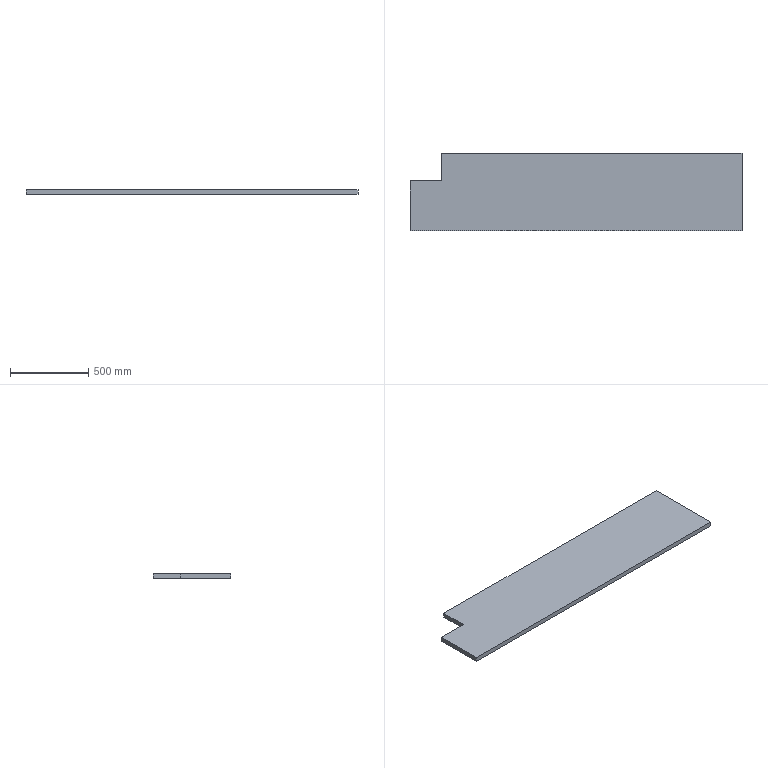Part | SolidWorks | features 3DProfileFeature 1, Extrusion 1, HoleWzd 1 | 1 solid | 24 faces | box 2118 x 492 x 30 mm | volume 30183108 mm3 | cylinder 8 | cone 8 | plane 8 | commonest cylinder face diameters 14 x8
STEP:
#1=CARTESIAN_POINT('',(918.,447.,8.));
#2=VERTEX_POINT('',#1);
#3=CARTESIAN_POINT('',(918.,447.,22.));
#4=VERTEX_POINT('',#3);
#5=CARTESIAN_POINT('',(918.,447.,15.));
#6=DIRECTION('',(0.,1.,0.));
#7=DIRECTION('',(0.,0.,1.));
#8=AXIS2_PLACEMENT_3D('',#5,#6,#7);
#9=CIRCLE('',#8,7.);
#10=EDGE_CURVE('',#2,#4,#9,.T.);
#11=ORIENTED_EDGE('',*,*,#10,.F.);
#12=CARTESIAN_POINT('',(918.,492.,8.));
#13=VERTEX_POINT('',#12);
#14=CARTESIAN_POINT('',(918.,492.,8.));
#15=DIRECTION('',(0.,1.,0.));
#16=VECTOR('',#15,1000.);
#17=LINE('',#14,#16);
#18=EDGE_CURVE('',#2,#13,#17,.T.);
#19=ORIENTED_EDGE('',*,*,#18,.T.);
#20=CARTESIAN_POINT('',(918.,492.,22.));
#21=VERTEX_POINT('',#20);
#22=CARTESIAN_POINT('',(918.,492.,15.));
#23=DIRECTION('',(0.,1.,0.));
#24=DIRECTION('',(0.,0.,1.));
#25=AXIS2_PLACEMENT_3D('',#22,#23,#24);
#26=CIRCLE('',#25,7.);
#27=EDGE_CURVE('',#13,#21,#26,.T.);
#28=ORIENTED_EDGE('',*,*,#27,.T.);
#29=CARTESIAN_POINT('',(918.,492.,22.));
#30=DIRECTION('',(0.,1.,0.));
#31=VECTOR('',#30,1000.);
#32=LINE('',#29,#31);
#33=EDGE_CURVE('',#4,#21,#32,.T.);
#34=ORIENTED_EDGE('',*,*,#33,.F.);
#35=EDGE_LOOP('',(#11,#19,#28,#34));
#36=FACE_OUTER_BOUND('',#35,.T.);
#37=CARTESIAN_POINT('',(918.,492.,15.));
#38=DIRECTION('',(0.,1.,0.));
#39=DIRECTION('',(0.,0.,1.));
#40=AXIS2_PLACEMENT_3D('',#37,#38,#39);
#41=CYLINDRICAL_SURFACE('',#40,7.);
#42=ADVANCED_FACE('',(#36),#41,.F.);
#43=CARTESIAN_POINT('',(918.,442.794,15.));
#44=VERTEX_POINT('',#43);
#45=CARTESIAN_POINT('',(918.,447.,22.));
#46=DIRECTION('',(0.,0.515,0.8572));
#47=VECTOR('',#46,1000.);
#48=LINE('',#45,#47);
#49=EDGE_CURVE('',#44,#4,#48,.T.);
#50=ORIENTED_EDGE('',*,*,#49,.F.);
#51=CARTESIAN_POINT('',(918.,447.,8.));
#52=DIRECTION('',(0.,0.515,-0.8572));
#53=VECTOR('',#52,1000.);
#54=LINE('',#51,#53);
#55=EDGE_CURVE('',#44,#2,#54,.T.);
#56=ORIENTED_EDGE('',*,*,#55,.T.);
#57=ORIENTED_EDGE('',*,*,#10,.T.);
#58=EDGE_LOOP('',(#50,#56,#57));
#59=FACE_OUTER_BOUND('',#58,.T.);
#60=CARTESIAN_POINT('',(918.,447.,15.));
#61=DIRECTION('',(0.,1.,0.));
#62=DIRECTION('',(0.,0.,1.));
#63=AXIS2_PLACEMENT_3D('',#60,#61,#62);
#64=CONICAL_SURFACE('',#63,7.,1.03);
#65=ADVANCED_FACE('',(#59),#64,.F.);
#66=CARTESIAN_POINT('',(1018.,447.,8.));
#67=VERTEX_POINT('',#66);
#68=CARTESIAN_POINT('',(1018.,447.,22.));
#69=VERTEX_POINT('',#68);
#70=CARTESIAN_POINT('',(1018.,447.,15.));
#71=DIRECTION('',(0.,1.,0.));
#72=DIRECTION('',(0.,0.,1.));
#73=AXIS2_PLACEMENT_3D('',#70,#71,#72);
#74=CIRCLE('',#73,7.);
#75=EDGE_CURVE('',#67,#69,#74,.T.);
#76=ORIENTED_EDGE('',*,*,#75,.F.);
#77=CARTESIAN_POINT('',(1018.,492.,8.));
#78=VERTEX_POINT('',#77);
#79=CARTESIAN_POINT('',(1018.,492.,8.));
#80=DIRECTION('',(0.,1.,0.));
#81=VECTOR('',#80,1000.);
#82=LINE('',#79,#81);
#83=EDGE_CURVE('',#67,#78,#82,.T.);
#84=ORIENTED_EDGE('',*,*,#83,.T.);
#85=CARTESIAN_POINT('',(1018.,492.,22.));
#86=VERTEX_POINT('',#85);
#87=CARTESIAN_POINT('',(1018.,492.,15.));
#88=DIRECTION('',(0.,1.,0.));
#89=DIRECTION('',(0.,0.,1.));
#90=AXIS2_PLACEMENT_3D('',#87,#88,#89);
#91=CIRCLE('',#90,7.);
#92=EDGE_CURVE('',#78,#86,#91,.T.);
#93=ORIENTED_EDGE('',*,*,#92,.T.);
#94=CARTESIAN_POINT('',(1018.,492.,22.));
#95=DIRECTION('',(0.,1.,0.));
#96=VECTOR('',#95,1000.);
#97=LINE('',#94,#96);
#98=EDGE_CURVE('',#69,#86,#97,.T.);
#99=ORIENTED_EDGE('',*,*,#98,.F.);
#100=EDGE_LOOP('',(#76,#84,#93,#99));
#101=FACE_OUTER_BOUND('',#100,.T.);
#102=CARTESIAN_POINT('',(1018.,492.,15.));
#103=DIRECTION('',(0.,1.,0.));
#104=DIRECTION('',(0.,0.,1.));
#105=AXIS2_PLACEMENT_3D('',#102,#103,#104);
#106=CYLINDRICAL_SURFACE('',#105,7.);
#107=ADVANCED_FACE('',(#101),#106,.F.);
#108=CARTESIAN_POINT('',(1018.,442.794,15.));
#109=VERTEX_POINT('',#108);
#110=CARTESIAN_POINT('',(1018.,447.,22.));
#111=DIRECTION('',(0.,0.515,0.8572));
#112=VECTOR('',#111,1000.);
#113=LINE('',#110,#112);
#114=EDGE_CURVE('',#109,#69,#113,.T.);
#115=ORIENTED_EDGE('',*,*,#114,.F.);
#116=CARTESIAN_POINT('',(1018.,447.,8.));
#117=DIRECTION('',(0.,0.515,-0.8572));
#118=VECTOR('',#117,1000.);
#119=LINE('',#116,#118);
#120=EDGE_CURVE('',#109,#67,#119,.T.);
#121=ORIENTED_EDGE('',*,*,#120,.T.);
#122=ORIENTED_EDGE('',*,*,#75,.T.);
#123=EDGE_LOOP('',(#115,#121,#122));
#124=FACE_OUTER_BOUND('',#123,.T.);
#125=CARTESIAN_POINT('',(1018.,447.,15.));
#126=DIRECTION('',(0.,1.,0.));
#127=DIRECTION('',(0.,0.,1.));
#128=AXIS2_PLACEMENT_3D('',#125,#126,#127);
#129=CONICAL_SURFACE('',#128,7.,1.03);
#130=ADVANCED_FACE('',(#124),#129,.F.);
#131=CARTESIAN_POINT('',(2068.,447.,8.));
#132=VERTEX_POINT('',#131);
#133=CARTESIAN_POINT('',(2068.,447.,22.));
#134=VERTEX_POINT('',#133);
#135=CARTESIAN_POINT('',(2068.,447.,15.));
#136=DIRECTION('',(0.,1.,0.));
#137=DIRECTION('',(0.,0.,1.));
#138=AXIS2_PLACEMENT_3D('',#135,#136,#137);
#139=CIRCLE('',#138,7.);
#140=EDGE_CURVE('',#132,#134,#139,.T.);
#141=ORIENTED_EDGE('',*,*,#140,.F.);
#142=CARTESIAN_POINT('',(2068.,492.,8.));
#143=VERTEX_POINT('',#142);
#144=CARTESIAN_POINT('',(2068.,492.,8.));
#145=DIRECTION('',(0.,1.,0.));
#146=VECTOR('',#145,1000.);
#147=LINE('',#144,#146);
#148=EDGE_CURVE('',#132,#143,#147,.T.);
#149=ORIENTED_EDGE('',*,*,#148,.T.);
#150=CARTESIAN_POINT('',(2068.,492.,22.));
#151=VERTEX_POINT('',#150);
#152=CARTESIAN_POINT('',(2068.,492.,15.));
#153=DIRECTION('',(0.,1.,0.));
#154=DIRECTION('',(0.,0.,1.));
#155=AXIS2_PLACEMENT_3D('',#152,#153,#154);
#156=CIRCLE('',#155,7.);
#157=EDGE_CURVE('',#143,#151,#156,.T.);
#158=ORIENTED_EDGE('',*,*,#157,.T.);
#159=CARTESIAN_POINT('',(2068.,492.,22.));
#160=DIRECTION('',(0.,1.,0.));
#161=VECTOR('',#160,1000.);
#162=LINE('',#159,#161);
#163=EDGE_CURVE('',#134,#151,#162,.T.);
#164=ORIENTED_EDGE('',*,*,#163,.F.);
#165=EDGE_LOOP('',(#141,#149,#158,#164));
#166=FACE_OUTER_BOUND('',#165,.T.);
#167=CARTESIAN_POINT('',(2068.,492.,15.));
#168=DIRECTION('',(0.,1.,0.));
#169=DIRECTION('',(0.,0.,1.));
#170=AXIS2_PLACEMENT_3D('',#167,#168,#169);
#171=CYLINDRICAL_SURFACE('',#170,7.);
#172=ADVANCED_FACE('',(#166),#171,.F.);
#173=CARTESIAN_POINT('',(2068.,442.794,15.));
#174=VERTEX_POINT('',#173);
#175=CARTESIAN_POINT('',(2068.,447.,22.));
#176=DIRECTION('',(0.,0.515,0.8572));
#177=VECTOR('',#176,1000.);
#178=LINE('',#175,#177);
#179=EDGE_CURVE('',#174,#134,#178,.T.);
#180=ORIENTED_EDGE('',*,*,#179,.F.);
#181=CARTESIAN_POINT('',(2068.,447.,8.));
#182=DIRECTION('',(0.,0.515,-0.8572));
#183=VECTOR('',#182,1000.);
#184=LINE('',#181,#183);
#185=EDGE_CURVE('',#174,#132,#184,.T.);
#186=ORIENTED_EDGE('',*,*,#185,.T.);
#187=ORIENTED_EDGE('',*,*,#140,.T.);
#188=EDGE_LOOP('',(#180,#186,#187));
#189=FACE_OUTER_BOUND('',#188,.T.);
#190=CARTESIAN_POINT('',(2068.,447.,15.));
#191=DIRECTION('',(0.,1.,0.));
#192=DIRECTION('',(0.,0.,1.));
#193=AXIS2_PLACEMENT_3D('',#190,#191,#192);
#194=CONICAL_SURFACE('',#193,7.,1.03);
#195=ADVANCED_FACE('',(#189),#194,.F.);
#196=CARTESIAN_POINT('',(1968.,447.,8.));
#197=VERTEX_POINT('',#196);
#198=CARTESIAN_POINT('',(1968.,447.,22.));
#199=VERTEX_POINT('',#198);
#200=CARTESIAN_POINT('',(1968.,447.,15.));
#201=DIRECTION('',(0.,1.,0.));
#202=DIRECTION('',(0.,0.,1.));
#203=AXIS2_PLACEMENT_3D('',#200,#201,#202);
#204=CIRCLE('',#203,7.);
#205=EDGE_CURVE('',#197,#199,#204,.T.);
#206=ORIENTED_EDGE('',*,*,#205,.F.);
#207=CARTESIAN_POINT('',(1968.,492.,8.));
#208=VERTEX_POINT('',#207);
#209=CARTESIAN_POINT('',(1968.,492.,8.));
#210=DIRECTION('',(0.,1.,0.));
#211=VECTOR('',#210,1000.);
#212=LINE('',#209,#211);
#213=EDGE_CURVE('',#197,#208,#212,.T.);
#214=ORIENTED_EDGE('',*,*,#213,.T.);
#215=CARTESIAN_POINT('',(1968.,492.,22.));
#216=VERTEX_POINT('',#215);
#217=CARTESIAN_POINT('',(1968.,492.,15.));
#218=DIRECTION('',(0.,1.,0.));
#219=DIRECTION('',(0.,0.,1.));
#220=AXIS2_PLACEMENT_3D('',#217,#218,#219);
#221=CIRCLE('',#220,7.);
#222=EDGE_CURVE('',#208,#216,#221,.T.);
#223=ORIENTED_EDGE('',*,*,#222,.T.);
#224=CARTESIAN_POINT('',(1968.,492.,22.));
#225=DIRECTION('',(0.,1.,0.));
#226=VECTOR('',#225,1000.);
#227=LINE('',#224,#226);
#228=EDGE_CURVE('',#199,#216,#227,.T.);
#229=ORIENTED_EDGE('',*,*,#228,.F.);
#230=EDGE_LOOP('',(#206,#214,#223,#229));
#231=FACE_OUTER_BOUND('',#230,.T.);
#232=CARTESIAN_POINT('',(1968.,492.,15.));
#233=DIRECTION('',(0.,1.,0.));
#234=DIRECTION('',(0.,0.,1.));
#235=AXIS2_PLACEMENT_3D('',#232,#233,#234);
#236=CYLINDRICAL_SURFACE('',#235,7.);
#237=ADVANCED_FACE('',(#231),#236,.F.);
#238=CARTESIAN_POINT('',(1968.,442.794,15.));
#239=VERTEX_POINT('',#238);
#240=CARTESIAN_POINT('',(1968.,447.,22.));
#241=DIRECTION('',(0.,0.515,0.8572));
#242=VECTOR('',#241,1000.);
#243=LINE('',#240,#242);
#244=EDGE_CURVE('',#239,#199,#243,.T.);
#245=ORIENTED_EDGE('',*,*,#244,.F.);
#246=CARTESIAN_POINT('',(1968.,447.,8.));
#247=DIRECTION('',(0.,0.515,-0.8572));
#248=VECTOR('',#247,1000.);
#249=LINE('',#246,#248);
#250=EDGE_CURVE('',#239,#197,#249,.T.);
#251=ORIENTED_EDGE('',*,*,#250,.T.);
#252=ORIENTED_EDGE('',*,*,#205,.T.);
#253=EDGE_LOOP('',(#245,#251,#252));
#254=FACE_OUTER_BOUND('',#253,.T.);
#255=CARTESIAN_POINT('',(1968.,447.,15.));
#256=DIRECTION('',(0.,1.,0.));
#257=DIRECTION('',(0.,0.,1.));
#258=AXIS2_PLACEMENT_3D('',#255,#256,#257);
#259=CONICAL_SURFACE('',#258,7.,1.03);
#260=ADVANCED_FACE('',(#254),#259,.F.);
#261=CARTESIAN_POINT('',(0.,317.,0.));
#262=VERTEX_POINT('',#261);
#263=CARTESIAN_POINT('',(0.,0.,0.));
#264=VERTEX_POINT('',#263);
#265=CARTESIAN_POINT('',(0.,0.,0.));
#266=DIRECTION('',(0.,-1.,0.));
#267=VECTOR('',#266,1000.);
#268=LINE('',#265,#267);
#269=EDGE_CURVE('',#262,#264,#268,.T.);
#270=ORIENTED_EDGE('',*,*,#269,.T.);
#271=CARTESIAN_POINT('',(0.,0.,30.));
#272=VERTEX_POINT('',#271);
#273=CARTESIAN_POINT('',(0.,0.,30.));
#274=DIRECTION('',(0.,0.,-1.));
#275=VECTOR('',#274,1000.);
#276=LINE('',#273,#275);
#277=EDGE_CURVE('',#272,#264,#276,.T.);
#278=ORIENTED_EDGE('',*,*,#277,.F.);
#279=CARTESIAN_POINT('',(0.,317.,30.));
#280=VERTEX_POINT('',#279);
#281=CARTESIAN_POINT('',(0.,0.,30.));
#282=DIRECTION('',(0.,-1.,0.));
#283=VECTOR('',#282,1000.);
#284=LINE('',#281,#283);
#285=EDGE_CURVE('',#280,#272,#284,.T.);
#286=ORIENTED_EDGE('',*,*,#285,.F.);
#287=CARTESIAN_POINT('',(0.,317.,30.));
#288=DIRECTION('',(0.,0.,-1.));
#289=VECTOR('',#288,1000.);
#290=LINE('',#287,#289);
#291=EDGE_CURVE('',#280,#262,#290,.T.);
#292=ORIENTED_EDGE('',*,*,#291,.T.);
#293=EDGE_LOOP('',(#270,#278,#286,#292));
#294=FACE_OUTER_BOUND('',#293,.T.);
#295=CARTESIAN_POINT('',(0.,0.,30.));
#296=DIRECTION('',(1.,0.,0.));
#297=DIRECTION('',(0.,0.,-1.));
#298=AXIS2_PLACEMENT_3D('',#295,#296,#297);
#299=PLANE('',#298);
#300=ADVANCED_FACE('',(#294),#299,.F.);
#301=CARTESIAN_POINT('',(2118.,0.,0.));
#302=VERTEX_POINT('',#301);
#303=CARTESIAN_POINT('',(0.,0.,0.));
#304=DIRECTION('',(1.,0.,0.));
#305=VECTOR('',#304,1000.);
#306=LINE('',#303,#305);
#307=EDGE_CURVE('',#264,#302,#306,.T.);
#308=ORIENTED_EDGE('',*,*,#307,.T.);
#309=CARTESIAN_POINT('',(2118.,0.,30.));
#310=VERTEX_POINT('',#309);
#311=CARTESIAN_POINT('',(2118.,0.,30.));
#312=DIRECTION('',(0.,0.,-1.));
#313=VECTOR('',#312,1000.);
#314=LINE('',#311,#313);
#315=EDGE_CURVE('',#310,#302,#314,.T.);
#316=ORIENTED_EDGE('',*,*,#315,.F.);
#317=CARTESIAN_POINT('',(0.,0.,30.));
#318=DIRECTION('',(1.,0.,0.));
#319=VECTOR('',#318,1000.);
#320=LINE('',#317,#319);
#321=EDGE_CURVE('',#272,#310,#320,.T.);
#322=ORIENTED_EDGE('',*,*,#321,.F.);
#323=ORIENTED_EDGE('',*,*,#277,.T.);
#324=EDGE_LOOP('',(#308,#316,#322,#323));
#325=FACE_OUTER_BOUND('',#324,.T.);
#326=CARTESIAN_POINT('',(0.,0.,30.));
#327=DIRECTION('',(0.,1.,0.));
#328=DIRECTION('',(0.,0.,1.));
#329=AXIS2_PLACEMENT_3D('',#326,#327,#328);
#330=PLANE('',#329);
#331=ADVANCED_FACE('',(#325),#330,.F.);
#332=CARTESIAN_POINT('',(2118.,492.,0.));
#333=VERTEX_POINT('',#332);
#334=CARTESIAN_POINT('',(2118.,0.,0.));
#335=DIRECTION('',(0.,1.,0.));
#336=VECTOR('',#335,1000.);
#337=LINE('',#334,#336);
#338=EDGE_CURVE('',#302,#333,#337,.T.);
#339=ORIENTED_EDGE('',*,*,#338,.T.);
#340=CARTESIAN_POINT('',(2118.,492.,30.));
#341=VERTEX_POINT('',#340);
#342=CARTESIAN_POINT('',(2118.,492.,30.));
#343=DIRECTION('',(0.,0.,-1.));
#344=VECTOR('',#343,1000.);
#345=LINE('',#342,#344);
#346=EDGE_CURVE('',#341,#333,#345,.T.);
#347=ORIENTED_EDGE('',*,*,#346,.F.);
#348=CARTESIAN_POINT('',(2118.,0.,30.));
#349=DIRECTION('',(0.,1.,0.));
#350=VECTOR('',#349,1000.);
#351=LINE('',#348,#350);
#352=EDGE_CURVE('',#310,#341,#351,.T.);
#353=ORIENTED_EDGE('',*,*,#352,.F.);
#354=ORIENTED_EDGE('',*,*,#315,.T.);
#355=EDGE_LOOP('',(#339,#347,#353,#354));
#356=FACE_OUTER_BOUND('',#355,.T.);
#357=CARTESIAN_POINT('',(2118.,0.,30.));
#358=DIRECTION('',(-1.,0.,0.));
#359=DIRECTION('',(0.,0.,1.));
#360=AXIS2_PLACEMENT_3D('',#357,#358,#359);
#361=PLANE('',#360);
#362=ADVANCED_FACE('',(#356),#361,.F.);
#363=CARTESIAN_POINT('',(918.,492.,15.));
#364=DIRECTION('',(0.,1.,0.));
#365=DIRECTION('',(0.,0.,1.));
#366=AXIS2_PLACEMENT_3D('',#363,#364,#365);
#367=CIRCLE('',#366,7.);
#368=EDGE_CURVE('',#21,#13,#367,.T.);
#369=ORIENTED_EDGE('',*,*,#368,.F.);
#370=ORIENTED_EDGE('',*,*,#27,.F.);
#371=EDGE_LOOP('',(#369,#370));
#372=FACE_BOUND('',#371,.T.);
#373=CARTESIAN_POINT('',(1018.,492.,15.));
#374=DIRECTION('',(0.,1.,0.));
#375=DIRECTION('',(0.,0.,1.));
#376=AXIS2_PLACEMENT_3D('',#373,#374,#375);
#377=CIRCLE('',#376,7.);
#378=EDGE_CURVE('',#86,#78,#377,.T.);
#379=ORIENTED_EDGE('',*,*,#378,.F.);
#380=ORIENTED_EDGE('',*,*,#92,.F.);
#381=EDGE_LOOP('',(#379,#380));
#382=FACE_BOUND('',#381,.T.);
#383=CARTESIAN_POINT('',(2068.,492.,15.));
#384=DIRECTION('',(0.,1.,0.));
#385=DIRECTION('',(0.,0.,1.));
#386=AXIS2_PLACEMENT_3D('',#383,#384,#385);
#387=CIRCLE('',#386,7.);
#388=EDGE_CURVE('',#151,#143,#387,.T.);
#389=ORIENTED_EDGE('',*,*,#388,.F.);
#390=ORIENTED_EDGE('',*,*,#157,.F.);
#391=EDGE_LOOP('',(#389,#390));
#392=FACE_BOUND('',#391,.T.);
#393=CARTESIAN_POINT('',(1968.,492.,15.));
#394=DIRECTION('',(0.,1.,0.));
#395=DIRECTION('',(0.,0.,1.));
#396=AXIS2_PLACEMENT_3D('',#393,#394,#395);
#397=CIRCLE('',#396,7.);
#398=EDGE_CURVE('',#216,#208,#397,.T.);
#399=ORIENTED_EDGE('',*,*,#398,.F.);
#400=ORIENTED_EDGE('',*,*,#222,.F.);
#401=EDGE_LOOP('',(#399,#400));
#402=FACE_BOUND('',#401,.T.);
#403=CARTESIAN_POINT('',(200.,492.,0.));
#404=VERTEX_POINT('',#403);
#405=CARTESIAN_POINT('',(200.,492.,0.));
#406=DIRECTION('',(-1.,0.,0.));
#407=VECTOR('',#406,1000.);
#408=LINE('',#405,#407);
#409=EDGE_CURVE('',#333,#404,#408,.T.);
#410=ORIENTED_EDGE('',*,*,#409,.T.);
#411=CARTESIAN_POINT('',(200.,492.,30.));
#412=VERTEX_POINT('',#411);
#413=CARTESIAN_POINT('',(200.,492.,30.));
#414=DIRECTION('',(0.,0.,-1.));
#415=VECTOR('',#414,1000.);
#416=LINE('',#413,#415);
#417=EDGE_CURVE('',#412,#404,#416,.T.);
#418=ORIENTED_EDGE('',*,*,#417,.F.);
#419=CARTESIAN_POINT('',(200.,492.,30.));
#420=DIRECTION('',(-1.,0.,0.));
#421=VECTOR('',#420,1000.);
#422=LINE('',#419,#421);
#423=EDGE_CURVE('',#341,#412,#422,.T.);
#424=ORIENTED_EDGE('',*,*,#423,.F.);
#425=ORIENTED_EDGE('',*,*,#346,.T.);
#426=EDGE_LOOP('',(#410,#418,#424,#425));
#427=FACE_OUTER_BOUND('',#426,.T.);
#428=CARTESIAN_POINT('',(200.,492.,30.));
#429=DIRECTION('',(0.,-1.,0.));
#430=DIRECTION('',(0.,0.,-1.));
#431=AXIS2_PLACEMENT_3D('',#428,#429,#430);
#432=PLANE('',#431);
#433=ADVANCED_FACE('',(#372,#382,#392,#402,#427),#432,.F.);
#434=CARTESIAN_POINT('',(200.,317.,0.));
#435=VERTEX_POINT('',#434);
#436=CARTESIAN_POINT('',(200.,317.,0.));
#437=DIRECTION('',(0.,-1.,0.));
#438=VECTOR('',#437,1000.);
#439=LINE('',#436,#438);
#440=EDGE_CURVE('',#404,#435,#439,.T.);
#441=ORIENTED_EDGE('',*,*,#440,.T.);
#442=CARTESIAN_POINT('',(200.,317.,30.));
#443=VERTEX_POINT('',#442);
#444=CARTESIAN_POINT('',(200.,317.,30.));
#445=DIRECTION('',(0.,0.,-1.));
#446=VECTOR('',#445,1000.);
#447=LINE('',#444,#446);
#448=EDGE_CURVE('',#443,#435,#447,.T.);
#449=ORIENTED_EDGE('',*,*,#448,.F.);
#450=CARTESIAN_POINT('',(200.,317.,30.));
#451=DIRECTION('',(0.,-1.,0.));
#452=VECTOR('',#451,1000.);
#453=LINE('',#450,#452);
#454=EDGE_CURVE('',#412,#443,#453,.T.);
#455=ORIENTED_EDGE('',*,*,#454,.F.);
#456=ORIENTED_EDGE('',*,*,#417,.T.);
#457=EDGE_LOOP('',(#441,#449,#455,#456));
#458=FACE_OUTER_BOUND('',#457,.T.);
#459=CARTESIAN_POINT('',(200.,317.,30.));
#460=DIRECTION('',(1.,0.,0.));
#461=DIRECTION('',(0.,0.,-1.));
#462=AXIS2_PLACEMENT_3D('',#459,#460,#461);
#463=PLANE('',#462);
#464=ADVANCED_FACE('',(#458),#463,.F.);
#465=CARTESIAN_POINT('',(0.,317.,0.));
#466=DIRECTION('',(-1.,0.,0.));
#467=VECTOR('',#466,1000.);
#468=LINE('',#465,#467);
#469=EDGE_CURVE('',#435,#262,#468,.T.);
#470=ORIENTED_EDGE('',*,*,#469,.T.);
#471=ORIENTED_EDGE('',*,*,#291,.F.);
#472=CARTESIAN_POINT('',(0.,317.,30.));
#473=DIRECTION('',(-1.,0.,0.));
#474=VECTOR('',#473,1000.);
#475=LINE('',#472,#474);
#476=EDGE_CURVE('',#443,#280,#475,.T.);
#477=ORIENTED_EDGE('',*,*,#476,.F.);
#478=ORIENTED_EDGE('',*,*,#448,.T.);
#479=EDGE_LOOP('',(#470,#471,#477,#478));
#480=FACE_OUTER_BOUND('',#479,.T.);
#481=CARTESIAN_POINT('',(0.,317.,30.));
#482=DIRECTION('',(0.,-1.,0.));
#483=DIRECTION('',(0.,0.,-1.));
#484=AXIS2_PLACEMENT_3D('',#481,#482,#483);
#485=PLANE('',#484);
#486=ADVANCED_FACE('',(#480),#485,.F.);
#487=ORIENTED_EDGE('',*,*,#285,.T.);
#488=ORIENTED_EDGE('',*,*,#321,.T.);
#489=ORIENTED_EDGE('',*,*,#352,.T.);
#490=ORIENTED_EDGE('',*,*,#423,.T.);
#491=ORIENTED_EDGE('',*,*,#454,.T.);
#492=ORIENTED_EDGE('',*,*,#476,.T.);
#493=EDGE_LOOP('',(#487,#488,#489,#490,#491,#492));
#494=FACE_OUTER_BOUND('',#493,.T.);
#495=CARTESIAN_POINT('',(0.,0.,30.));
#496=DIRECTION('',(0.,0.,-1.));
#497=DIRECTION('',(-1.,0.,0.));
#498=AXIS2_PLACEMENT_3D('',#495,#496,#497);
#499=PLANE('',#498);
#500=ADVANCED_FACE('',(#494),#499,.F.);
#501=ORIENTED_EDGE('',*,*,#269,.F.);
#502=ORIENTED_EDGE('',*,*,#469,.F.);
#503=ORIENTED_EDGE('',*,*,#440,.F.);
#504=ORIENTED_EDGE('',*,*,#409,.F.);
#505=ORIENTED_EDGE('',*,*,#338,.F.);
#506=ORIENTED_EDGE('',*,*,#307,.F.);
#507=EDGE_LOOP('',(#501,#502,#503,#504,#505,#506));
#508=FACE_OUTER_BOUND('',#507,.T.);
#509=CARTESIAN_POINT('',(0.,0.,0.));
#510=DIRECTION('',(0.,0.,-1.));
#511=DIRECTION('',(-1.,0.,0.));
#512=AXIS2_PLACEMENT_3D('',#509,#510,#511);
#513=PLANE('',#512);
#514=ADVANCED_FACE('',(#508),#513,.T.);
#515=ORIENTED_EDGE('',*,*,#250,.F.);
#516=ORIENTED_EDGE('',*,*,#244,.T.);
#517=CARTESIAN_POINT('',(1968.,447.,15.));
#518=DIRECTION('',(0.,1.,0.));
#519=DIRECTION('',(0.,0.,1.));
#520=AXIS2_PLACEMENT_3D('',#517,#518,#519);
#521=CIRCLE('',#520,7.);
#522=EDGE_CURVE('',#199,#197,#521,.T.);
#523=ORIENTED_EDGE('',*,*,#522,.T.);
#524=EDGE_LOOP('',(#515,#516,#523));
#525=FACE_OUTER_BOUND('',#524,.T.);
#526=CARTESIAN_POINT('',(1968.,447.,15.));
#527=DIRECTION('',(0.,1.,0.));
#528=DIRECTION('',(0.,0.,1.));
#529=AXIS2_PLACEMENT_3D('',#526,#527,#528);
#530=CONICAL_SURFACE('',#529,7.,1.03);
#531=ADVANCED_FACE('',(#525),#530,.F.);
#532=ORIENTED_EDGE('',*,*,#213,.F.);
#533=ORIENTED_EDGE('',*,*,#522,.F.);
#534=ORIENTED_EDGE('',*,*,#228,.T.);
#535=ORIENTED_EDGE('',*,*,#398,.T.);
#536=EDGE_LOOP('',(#532,#533,#534,#535));
#537=FACE_OUTER_BOUND('',#536,.T.);
#538=CARTESIAN_POINT('',(1968.,492.,15.));
#539=DIRECTION('',(0.,1.,0.));
#540=DIRECTION('',(0.,0.,1.));
#541=AXIS2_PLACEMENT_3D('',#538,#539,#540);
#542=CYLINDRICAL_SURFACE('',#541,7.);
#543=ADVANCED_FACE('',(#537),#542,.F.);
#544=ORIENTED_EDGE('',*,*,#185,.F.);
#545=ORIENTED_EDGE('',*,*,#179,.T.);
#546=CARTESIAN_POINT('',(2068.,447.,15.));
#547=DIRECTION('',(0.,1.,0.));
#548=DIRECTION('',(0.,0.,1.));
#549=AXIS2_PLACEMENT_3D('',#546,#547,#548);
#550=CIRCLE('',#549,7.);
#551=EDGE_CURVE('',#134,#132,#550,.T.);
#552=ORIENTED_EDGE('',*,*,#551,.T.);
#553=EDGE_LOOP('',(#544,#545,#552));
#554=FACE_OUTER_BOUND('',#553,.T.);
#555=CARTESIAN_POINT('',(2068.,447.,15.));
#556=DIRECTION('',(0.,1.,0.));
#557=DIRECTION('',(0.,0.,1.));
#558=AXIS2_PLACEMENT_3D('',#555,#556,#557);
#559=CONICAL_SURFACE('',#558,7.,1.03);
#560=ADVANCED_FACE('',(#554),#559,.F.);
#561=ORIENTED_EDGE('',*,*,#148,.F.);
#562=ORIENTED_EDGE('',*,*,#551,.F.);
#563=ORIENTED_EDGE('',*,*,#163,.T.);
#564=ORIENTED_EDGE('',*,*,#388,.T.);
#565=EDGE_LOOP('',(#561,#562,#563,#564));
#566=FACE_OUTER_BOUND('',#565,.T.);
#567=CARTESIAN_POINT('',(2068.,492.,15.));
#568=DIRECTION('',(0.,1.,0.));
#569=DIRECTION('',(0.,0.,1.));
#570=AXIS2_PLACEMENT_3D('',#567,#568,#569);
#571=CYLINDRICAL_SURFACE('',#570,7.);
#572=ADVANCED_FACE('',(#566),#571,.F.);
#573=ORIENTED_EDGE('',*,*,#120,.F.);
#574=ORIENTED_EDGE('',*,*,#114,.T.);
#575=CARTESIAN_POINT('',(1018.,447.,15.));
#576=DIRECTION('',(0.,1.,0.));
#577=DIRECTION('',(0.,0.,1.));
#578=AXIS2_PLACEMENT_3D('',#575,#576,#577);
#579=CIRCLE('',#578,7.);
#580=EDGE_CURVE('',#69,#67,#579,.T.);
#581=ORIENTED_EDGE('',*,*,#580,.T.);
#582=EDGE_LOOP('',(#573,#574,#581));
#583=FACE_OUTER_BOUND('',#582,.T.);
#584=CARTESIAN_POINT('',(1018.,447.,15.));
#585=DIRECTION('',(0.,1.,0.));
#586=DIRECTION('',(0.,0.,1.));
#587=AXIS2_PLACEMENT_3D('',#584,#585,#586);
#588=CONICAL_SURFACE('',#587,7.,1.03);
#589=ADVANCED_FACE('',(#583),#588,.F.);
#590=ORIENTED_EDGE('',*,*,#83,.F.);
#591=ORIENTED_EDGE('',*,*,#580,.F.);
#592=ORIENTED_EDGE('',*,*,#98,.T.);
#593=ORIENTED_EDGE('',*,*,#378,.T.);
#594=EDGE_LOOP('',(#590,#591,#592,#593));
#595=FACE_OUTER_BOUND('',#594,.T.);
#596=CARTESIAN_POINT('',(1018.,492.,15.));
#597=DIRECTION('',(0.,1.,0.));
#598=DIRECTION('',(0.,0.,1.));
#599=AXIS2_PLACEMENT_3D('',#596,#597,#598);
#600=CYLINDRICAL_SURFACE('',#599,7.);
#601=ADVANCED_FACE('',(#595),#600,.F.);
#602=ORIENTED_EDGE('',*,*,#55,.F.);
#603=ORIENTED_EDGE('',*,*,#49,.T.);
#604=CARTESIAN_POINT('',(918.,447.,15.));
#605=DIRECTION('',(0.,1.,0.));
#606=DIRECTION('',(0.,0.,1.));
#607=AXIS2_PLACEMENT_3D('',#604,#605,#606);
#608=CIRCLE('',#607,7.);
#609=EDGE_CURVE('',#4,#2,#608,.T.);
#610=ORIENTED_EDGE('',*,*,#609,.T.);
#611=EDGE_LOOP('',(#602,#603,#610));
#612=FACE_OUTER_BOUND('',#611,.T.);
#613=CARTESIAN_POINT('',(918.,447.,15.));
#614=DIRECTION('',(0.,1.,0.));
#615=DIRECTION('',(0.,0.,1.));
#616=AXIS2_PLACEMENT_3D('',#613,#614,#615);
#617=CONICAL_SURFACE('',#616,7.,1.03);
#618=ADVANCED_FACE('',(#612),#617,.F.);
#619=ORIENTED_EDGE('',*,*,#18,.F.);
#620=ORIENTED_EDGE('',*,*,#609,.F.);
#621=ORIENTED_EDGE('',*,*,#33,.T.);
#622=ORIENTED_EDGE('',*,*,#368,.T.);
#623=EDGE_LOOP('',(#619,#620,#621,#622));
#624=FACE_OUTER_BOUND('',#623,.T.);
#625=CARTESIAN_POINT('',(918.,492.,15.));
#626=DIRECTION('',(0.,1.,0.));
#627=DIRECTION('',(0.,0.,1.));
#628=AXIS2_PLACEMENT_3D('',#625,#626,#627);
#629=CYLINDRICAL_SURFACE('',#628,7.);
#630=ADVANCED_FACE('',(#624),#629,.F.);
#631=CLOSED_SHELL('',(#42,#65,#107,#130,#172,#195,#237,#260,#300,#331,#362,#433,#464,#486,#500,#514,#531,#543,#560,#572,#589,#601,#618,#630));
#632=MANIFOLD_SOLID_BREP('',#631);
#633=CARTESIAN_POINT('',(0.,0.,0.));
#634=DIRECTION('',(0.,0.,1.));
#635=DIRECTION('',(1.,0.,0.));
#636=AXIS2_PLACEMENT_3D('',#633,#634,#635);
#637=(LENGTH_UNIT()NAMED_UNIT(*)SI_UNIT(.MILLI.,.METRE.));
#638=UNCERTAINTY_MEASURE_WITH_UNIT(LENGTH_MEASURE(0.00001),#637,'','');
#639=(NAMED_UNIT(*)PLANE_ANGLE_UNIT()SI_UNIT($,.RADIAN.));
#640=(NAMED_UNIT(*)SI_UNIT($,.STERADIAN.)SOLID_ANGLE_UNIT());
#641=(GEOMETRIC_REPRESENTATION_CONTEXT(3)GLOBAL_UNCERTAINTY_ASSIGNED_CONTEXT((#638))GLOBAL_UNIT_ASSIGNED_CONTEXT((#637,#639,#640))REPRESENTATION_CONTEXT('',''));
#642=ADVANCED_BREP_SHAPE_REPRESENTATION('',(#632,#636),#641);